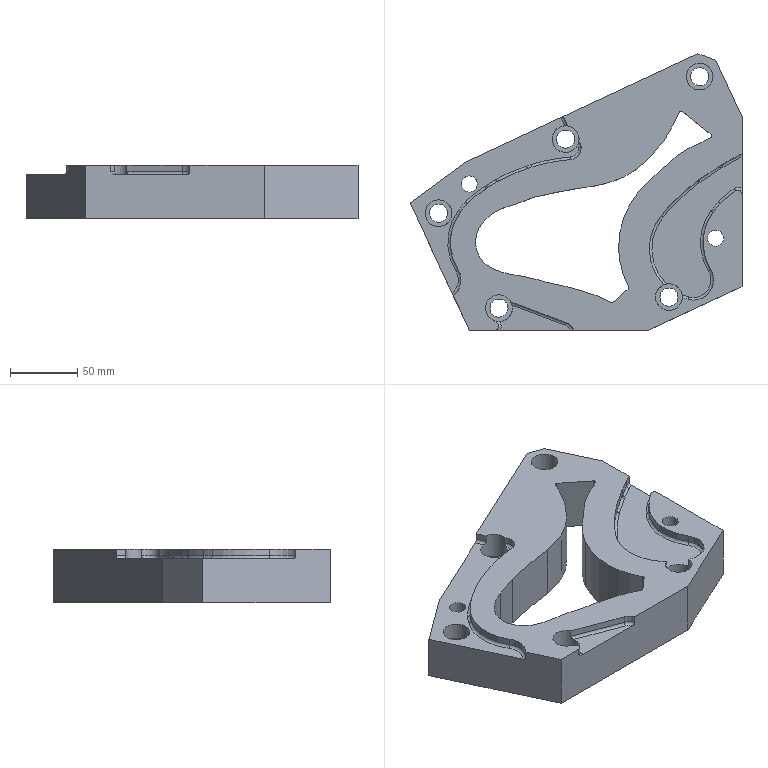Part | NX | features 23 2 | 1 solid | 119 faces | box 247.012 x 205.729 x 40 mm | volume 1008365 mm3 | cylinder 55 | plane 27 | spline 22 | torus 15 | commonest cylinder face diameters 4 x5 13.5 x5 20 x5 3 x4 6 x2 12.001 x2